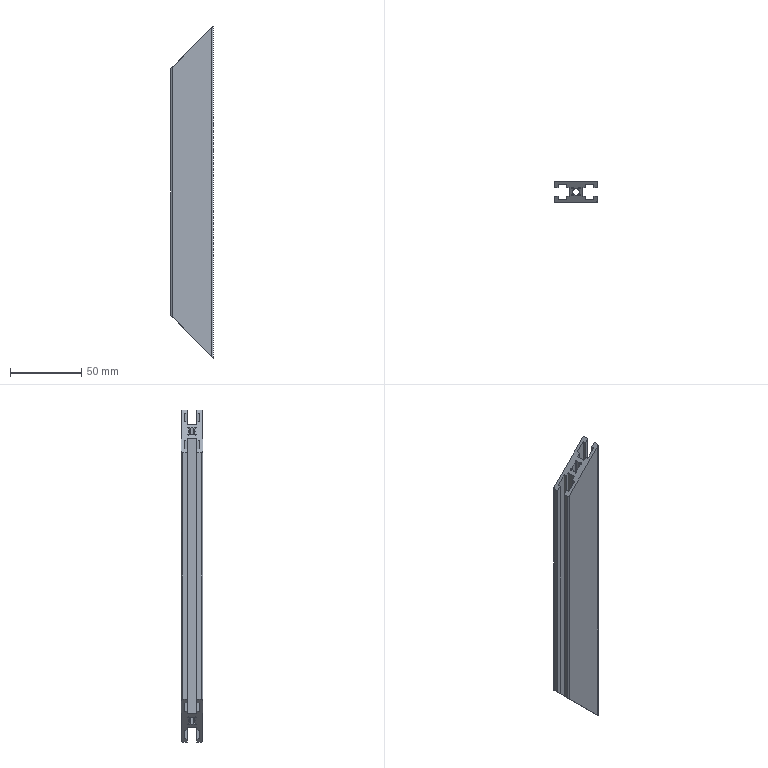Part | NX | features BREP 1 | 1 solid | 91 faces | box 30 x 15 x 233.5 mm | volume 48773 mm3 | plane 46 | cylinder 41 | cone 4 | commonest cylinder face diameters 5 x31 1 x6 2 x4